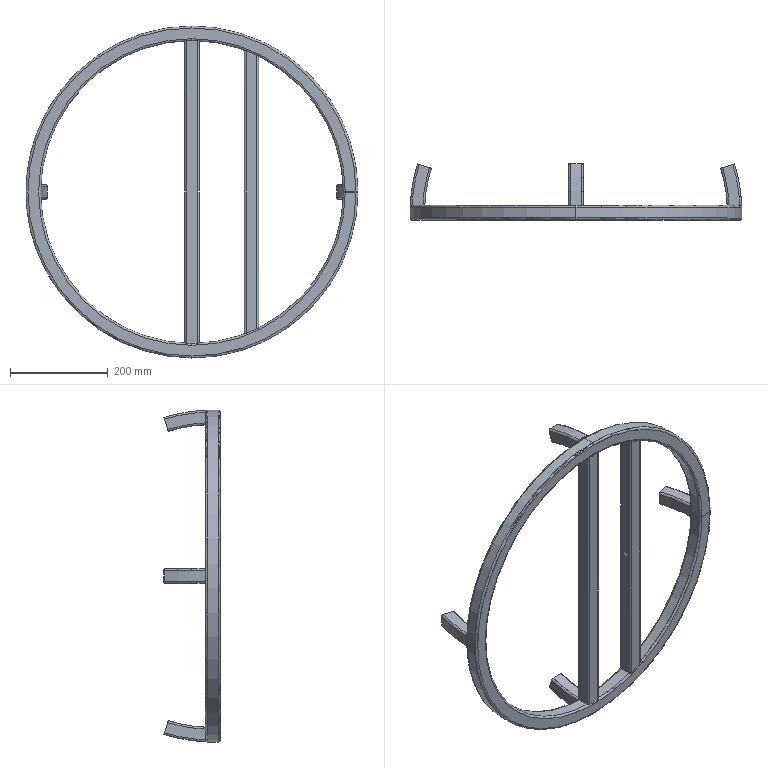Part | SolidWorks | features ICE 3, WeldMemberFeat 2, CirPattern 1, WeldmentFeature 1 | 7 solids | 155 faces | box 680 x 115 x 680 mm | volume 760065 mm3 | torus 56 | cylinder 53 | plane 46 | commonest cylinder face diameters 620 x12 4 x8 8 x8 624 x7 676 x7 680 x7